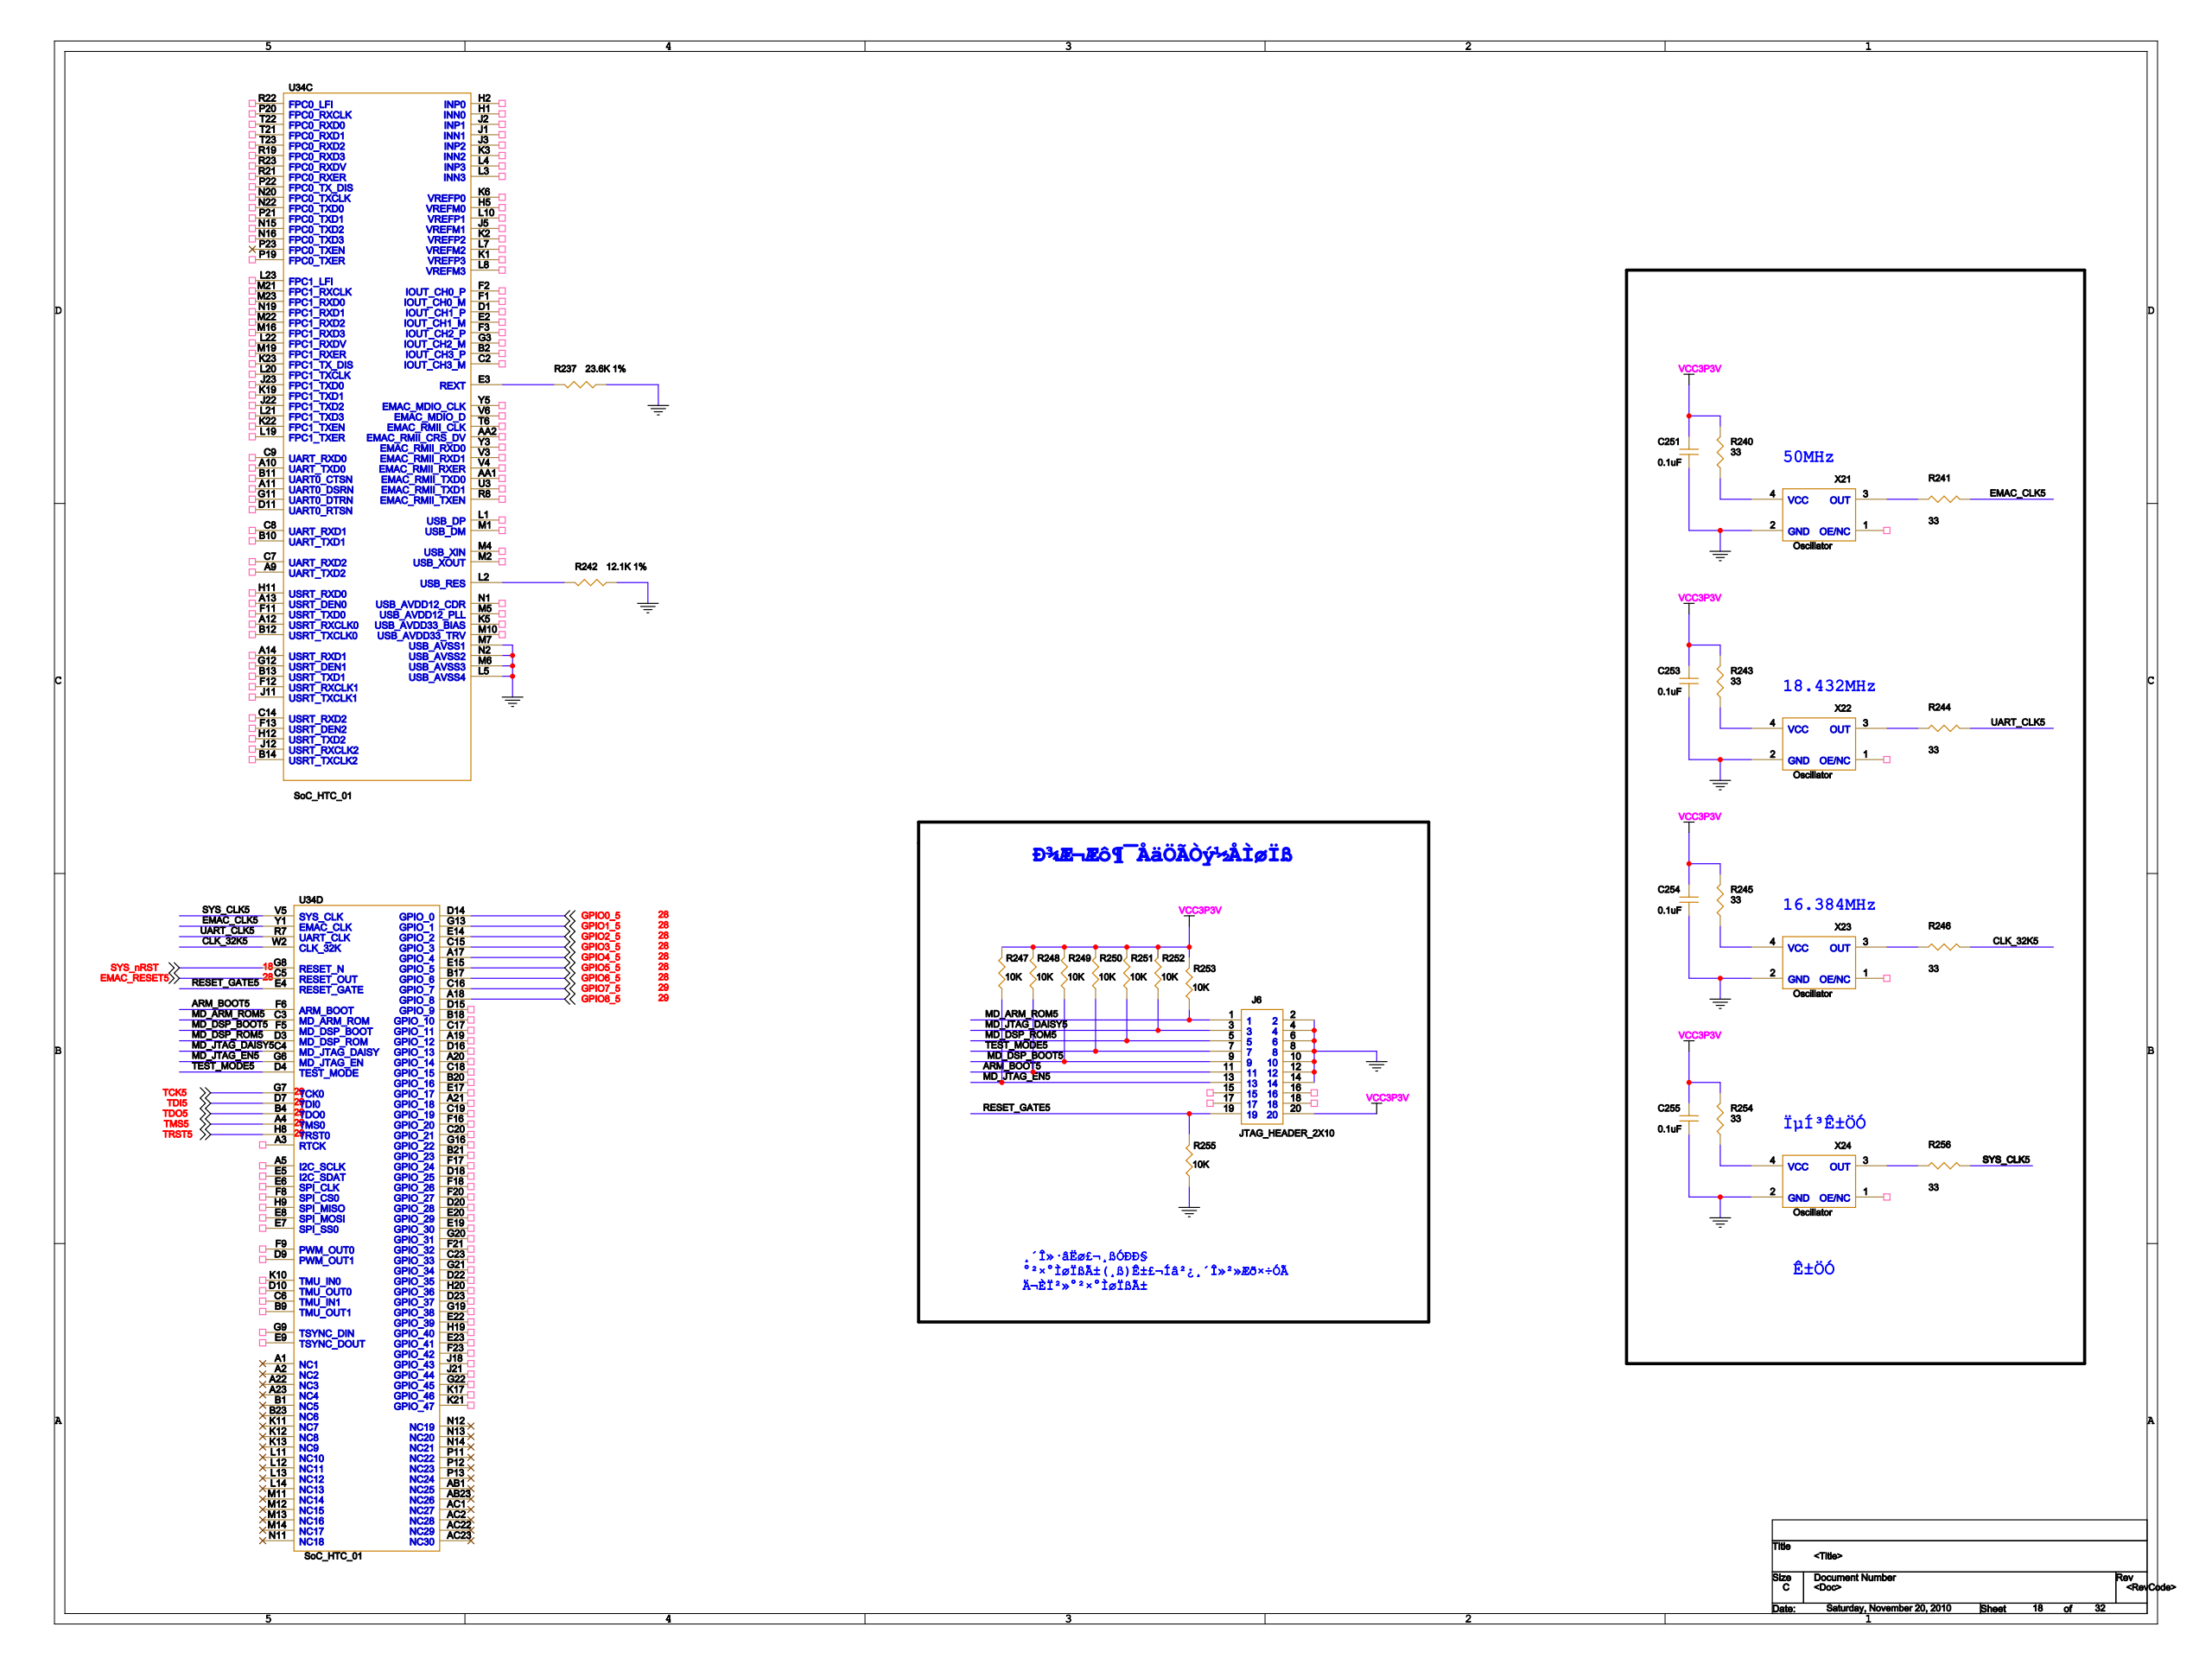Circuit board | Cadence Allegro | 1001 parts | 1318 nets | one sheet of the schematic
Parts on this sheet (reference | value | footprint):
C251 | 0.1uF | 0603
C253 | 0.1uF | 0603
C254 | 0.1uF | 0603
C255 | 0.1uF | 0603
J6 | JTAG_HEADER_2X10 | JTAG_HEADER_2X10
R237 | 23.6K 1% | 0603
R240 | 33 | 0603
R241 | 33 | 0603
R242 | 12.1K 1% | 0603
R243 | 33 | 0603
R244 | 33 | 0603
R245 | 33 | 0603
R246 | 33 | 0603
R247 | 10K | 0603
R248 | 10K | 0603
R249 | 10K | 0603
R250 | 10K | 0603
R251 | 10K | 0603
R252 | 10K | 0603
R253 | 10K | 0603
R254 | 33 | 0603
R255 | 10K | 0603
R256 | 33 | 0603
U34 | SoC_HTC_01 | L529_XIN
X21 | Oscillator | OSC_5_7
X22 | Oscillator | OSC_5_7
X23 | Oscillator | OSC_5_7
X24 | Oscillator | OSC_5_7
Nets of these parts (net: part-pin ...):
GPIO8_5: U34-A18
GPIO6_5: U34-B17
GPIO3_5: U34-C15
GPIO4_5: U34-A17
GPIO1_5: U34-G13
GPIO7_5: U34-C16
TRST5: U34-H8
TCK5: U34-G7
TDI5: U34-D7
TDO5: U34-B4
TMS5: U34-A4
GPIO5_5: U34-E15
GPIO0_5: U34-D14
GPIO2_5: U34-E14
EMAC_RESET5: U34-C5
GND: C251-2 C253-2 C254-2 C255-2 J6-2 J6-4 J6-6 J6-8 J6-10 J6-12 J6-14 R237-1 R242-1 R255-1 X21-2 X22-2 X23-2 X24-2 U34-L5 U34-M6 U34-M7 U34-N2
VCC3P3V: C251-1 C253-1 C254-1 C255-1 J6-20 R240-2 R243-2 R245-2 R247-2 R248-2 R249-2 R250-2 R251-2 R252-2 R253-2 R254-2 U34-J6
N16886604: R237-2 U34-E3
N16886816: R242-2 U34-L2
ARM_BOOT5: J6-11 R248-1 U34-F6
CLK_32K5: R246-2 U34-W2
EMAC_CLK5: R241-2 U34-Y1
MD_ARM_ROM5: J6-1 R253-1 U34-C3
MD_DSP_BOOT5: J6-9 R249-1 U34-F5
MD_DSP_ROM5: J6-5 R251-1 U34-D3
MD_JTAG_DAISY5: J6-3 R252-1 U34-C4
MD_JTAG_EN5: J6-13 R247-1 U34-G6
RESET_GATE5: J6-19 R255-2 U34-E4
SYS_CLK_16886399: R256-2 U34-V5
TEST_MODE5: J6-7 R250-1 U34-D4
UART_CLK5: R244-2 U34-R7
N16887334: R240-1 X21-4
N16887310: R241-1 X21-3
N16887324: R243-1 X22-4
N16887342: R244-1 X22-3
N16886357: R245-1 X23-4
N16886389: R246-1 X23-3
N16886368: R254-1 X24-4
N16886418: R256-1 X24-3